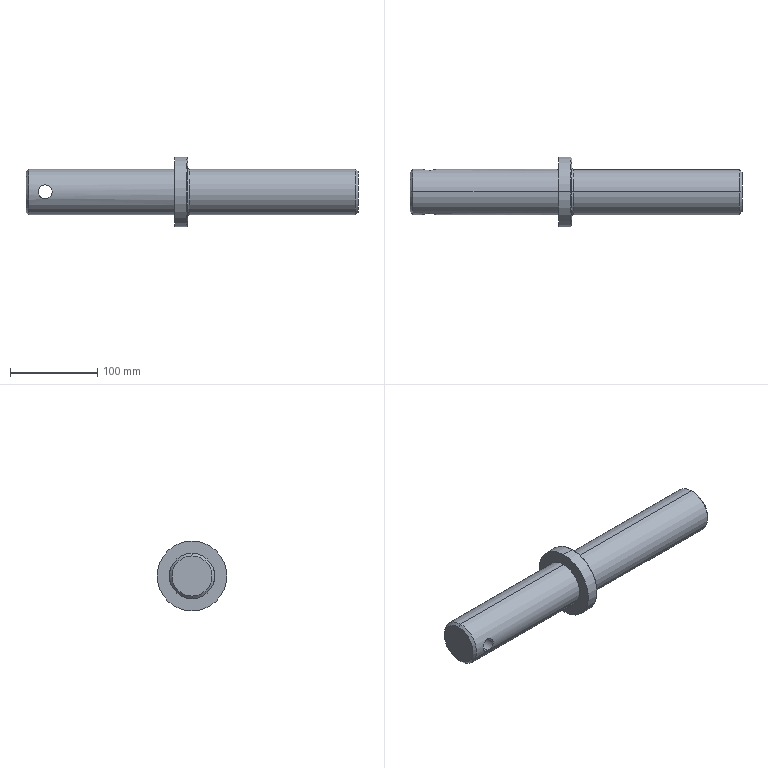Part | NX | features BREP 1 | 1 solid | 20 faces | box 380 x 80 x 80 mm | volume 838833 mm3 | cylinder 8 | cone 6 | plane 4 | torus 2 | commonest cylinder face diameters 52 x4 16 x2 80 x2
STEP:
#1=CARTESIAN_POINT('',(22.,-24.787,-7.85));
#2=VERTEX_POINT('',#1);
#3=CARTESIAN_POINT('',(22.,-24.689,8.15));
#4=VERTEX_POINT('',#3);
#5=CARTESIAN_POINT('',(22.,-24.787,-7.85));
#6=CARTESIAN_POINT('',(19.872,-24.787,-7.85));
#7=CARTESIAN_POINT('',(15.748,-25.421,-6.116));
#8=CARTESIAN_POINT('',(13.125,-26.307,0.145));
#9=CARTESIAN_POINT('',(15.749,-25.348,6.42));
#10=CARTESIAN_POINT('',(19.872,-24.689,8.15));
#11=CARTESIAN_POINT('',(22.,-24.689,8.15));
#12=B_SPLINE_CURVE_WITH_KNOTS('',3,(#5,#6,#7,#8,#9,#10,#11),.UNSPECIFIED.,.F.,.F.,(4,1,1,1,4),(0.,0.006289,0.01258,0.01887,0.02516),.UNSPECIFIED.);
#13=EDGE_CURVE('',#2,#4,#12,.T.);
#14=ORIENTED_EDGE('',*,*,#13,.F.);
#15=CARTESIAN_POINT('',(22.,24.787,-7.85));
#16=VERTEX_POINT('',#15);
#17=CARTESIAN_POINT('',(22.,-50.,-7.85));
#18=DIRECTION('',(0.,1.,0.));
#19=VECTOR('',#18,1000.);
#20=LINE('',#17,#19);
#21=EDGE_CURVE('',#2,#16,#20,.T.);
#22=ORIENTED_EDGE('',*,*,#21,.T.);
#23=CARTESIAN_POINT('',(22.,24.689,8.15));
#24=VERTEX_POINT('',#23);
#25=CARTESIAN_POINT('',(22.,24.689,8.15));
#26=CARTESIAN_POINT('',(19.872,24.689,8.15));
#27=CARTESIAN_POINT('',(15.753,25.347,6.416));
#28=CARTESIAN_POINT('',(13.126,26.307,0.1709));
#29=CARTESIAN_POINT('',(15.744,25.422,-6.119));
#30=CARTESIAN_POINT('',(19.872,24.787,-7.85));
#31=CARTESIAN_POINT('',(22.,24.787,-7.85));
#32=B_SPLINE_CURVE_WITH_KNOTS('',3,(#25,#26,#27,#28,#29,#30,#31),.UNSPECIFIED.,.F.,.F.,(4,1,1,1,4),(0.,0.006289,0.01258,0.01887,0.02516),.UNSPECIFIED.);
#33=EDGE_CURVE('',#24,#16,#32,.T.);
#34=ORIENTED_EDGE('',*,*,#33,.F.);
#35=CARTESIAN_POINT('',(22.,-50.,8.15));
#36=DIRECTION('',(0.,1.,0.));
#37=VECTOR('',#36,1000.);
#38=LINE('',#35,#37);
#39=EDGE_CURVE('',#4,#24,#38,.T.);
#40=ORIENTED_EDGE('',*,*,#39,.F.);
#41=EDGE_LOOP('',(#14,#22,#34,#40));
#42=FACE_BOUND('',#41,.T.);
#43=CARTESIAN_POINT('',(22.,-50.,0.1503));
#44=DIRECTION('',(0.,1.,0.));
#45=DIRECTION('',(0.,0.,-1.));
#46=AXIS2_PLACEMENT_3D('',#43,#44,#45);
#47=CYLINDRICAL_SURFACE('',#46,8.);
#48=ADVANCED_FACE('',(#42),#47,.F.);
#49=CARTESIAN_POINT('',(380.,0.,-23.));
#50=VERTEX_POINT('',#49);
#51=CARTESIAN_POINT('',(380.,0.,23.));
#52=VERTEX_POINT('',#51);
#53=CARTESIAN_POINT('',(380.,0.,0.));
#54=DIRECTION('',(1.,0.,0.));
#55=DIRECTION('',(0.,0.,1.));
#56=AXIS2_PLACEMENT_3D('',#53,#54,#55);
#57=CIRCLE('',#56,23.);
#58=EDGE_CURVE('',#50,#52,#57,.T.);
#59=ORIENTED_EDGE('',*,*,#58,.F.);
#60=CARTESIAN_POINT('',(377.,0.,-26.));
#61=VERTEX_POINT('',#60);
#62=CARTESIAN_POINT('',(377.,0.,-26.));
#63=DIRECTION('',(-0.7071,0.,-0.7071));
#64=VECTOR('',#63,1000.);
#65=LINE('',#62,#64);
#66=EDGE_CURVE('',#50,#61,#65,.T.);
#67=ORIENTED_EDGE('',*,*,#66,.T.);
#68=CARTESIAN_POINT('',(377.,0.,26.));
#69=VERTEX_POINT('',#68);
#70=CARTESIAN_POINT('',(377.,0.,0.));
#71=DIRECTION('',(-1.,0.,0.));
#72=DIRECTION('',(0.,0.,1.));
#73=AXIS2_PLACEMENT_3D('',#70,#71,#72);
#74=CIRCLE('',#73,26.);
#75=EDGE_CURVE('',#69,#61,#74,.T.);
#76=ORIENTED_EDGE('',*,*,#75,.F.);
#77=CARTESIAN_POINT('',(377.,0.,26.));
#78=DIRECTION('',(-0.7071,0.,0.7071));
#79=VECTOR('',#78,1000.);
#80=LINE('',#77,#79);
#81=EDGE_CURVE('',#52,#69,#80,.T.);
#82=ORIENTED_EDGE('',*,*,#81,.F.);
#83=EDGE_LOOP('',(#59,#67,#76,#82));
#84=FACE_BOUND('',#83,.T.);
#85=CARTESIAN_POINT('',(377.,0.,0.));
#86=DIRECTION('',(-1.,0.,0.));
#87=DIRECTION('',(0.,0.,-1.));
#88=AXIS2_PLACEMENT_3D('',#85,#86,#87);
#89=CONICAL_SURFACE('',#88,26.,0.7854);
#90=ADVANCED_FACE('',(#84),#89,.T.);
#91=CARTESIAN_POINT('',(0.,0.,23.));
#92=VERTEX_POINT('',#91);
#93=CARTESIAN_POINT('',(0.,0.,-23.));
#94=VERTEX_POINT('',#93);
#95=CARTESIAN_POINT('',(0.,0.,0.));
#96=DIRECTION('',(-1.,0.,0.));
#97=DIRECTION('',(0.,0.,-1.));
#98=AXIS2_PLACEMENT_3D('',#95,#96,#97);
#99=CIRCLE('',#98,23.);
#100=EDGE_CURVE('',#92,#94,#99,.T.);
#101=ORIENTED_EDGE('',*,*,#100,.F.);
#102=CARTESIAN_POINT('',(3.,0.,26.));
#103=VERTEX_POINT('',#102);
#104=CARTESIAN_POINT('',(0.,0.,23.));
#105=DIRECTION('',(0.7071,0.,0.7071));
#106=VECTOR('',#105,1000.);
#107=LINE('',#104,#106);
#108=EDGE_CURVE('',#103,#92,#107,.F.);
#109=ORIENTED_EDGE('',*,*,#108,.F.);
#110=CARTESIAN_POINT('',(3.,0.,-26.));
#111=VERTEX_POINT('',#110);
#112=CARTESIAN_POINT('',(3.,0.,0.));
#113=DIRECTION('',(1.,0.,0.));
#114=DIRECTION('',(0.,0.,-1.));
#115=AXIS2_PLACEMENT_3D('',#112,#113,#114);
#116=CIRCLE('',#115,26.);
#117=EDGE_CURVE('',#111,#103,#116,.T.);
#118=ORIENTED_EDGE('',*,*,#117,.F.);
#119=CARTESIAN_POINT('',(0.,0.,-23.));
#120=DIRECTION('',(0.7071,0.,-0.7071));
#121=VECTOR('',#120,1000.);
#122=LINE('',#119,#121);
#123=EDGE_CURVE('',#111,#94,#122,.F.);
#124=ORIENTED_EDGE('',*,*,#123,.T.);
#125=EDGE_LOOP('',(#101,#109,#118,#124));
#126=FACE_BOUND('',#125,.T.);
#127=CARTESIAN_POINT('',(0.,0.,0.));
#128=DIRECTION('',(1.,0.,0.));
#129=DIRECTION('',(0.,0.,1.));
#130=AXIS2_PLACEMENT_3D('',#127,#128,#129);
#131=CONICAL_SURFACE('',#130,23.,0.7854);
#132=ADVANCED_FACE('',(#126),#131,.T.);
#133=CARTESIAN_POINT('',(185.,0.,-28.));
#134=VERTEX_POINT('',#133);
#135=CARTESIAN_POINT('',(185.,0.,28.));
#136=VERTEX_POINT('',#135);
#137=CARTESIAN_POINT('',(185.,0.,0.));
#138=DIRECTION('',(-1.,0.,0.));
#139=DIRECTION('',(0.,0.,1.));
#140=AXIS2_PLACEMENT_3D('',#137,#138,#139);
#141=CIRCLE('',#140,28.);
#142=EDGE_CURVE('',#134,#136,#141,.T.);
#143=ORIENTED_EDGE('',*,*,#142,.F.);
#144=CARTESIAN_POINT('',(187.,0.,-26.));
#145=VERTEX_POINT('',#144);
#146=CARTESIAN_POINT('',(187.,0.,-28.));
#147=DIRECTION('',(0.,1.,0.));
#148=DIRECTION('',(0.,0.,1.));
#149=AXIS2_PLACEMENT_3D('',#146,#147,#148);
#150=CIRCLE('',#149,2.);
#151=EDGE_CURVE('',#134,#145,#150,.T.);
#152=ORIENTED_EDGE('',*,*,#151,.T.);
#153=CARTESIAN_POINT('',(187.,0.,26.));
#154=VERTEX_POINT('',#153);
#155=CARTESIAN_POINT('',(187.,0.,0.));
#156=DIRECTION('',(1.,0.,0.));
#157=DIRECTION('',(0.,0.,1.));
#158=AXIS2_PLACEMENT_3D('',#155,#156,#157);
#159=CIRCLE('',#158,26.);
#160=EDGE_CURVE('',#154,#145,#159,.T.);
#161=ORIENTED_EDGE('',*,*,#160,.F.);
#162=CARTESIAN_POINT('',(187.,0.,28.));
#163=DIRECTION('',(0.,-1.,0.));
#164=DIRECTION('',(0.,0.,-1.));
#165=AXIS2_PLACEMENT_3D('',#162,#163,#164);
#166=CIRCLE('',#165,2.);
#167=EDGE_CURVE('',#136,#154,#166,.T.);
#168=ORIENTED_EDGE('',*,*,#167,.F.);
#169=EDGE_LOOP('',(#143,#152,#161,#168));
#170=FACE_BOUND('',#169,.T.);
#171=CARTESIAN_POINT('',(187.,0.,0.));
#172=DIRECTION('',(-1.,0.,0.));
#173=DIRECTION('',(0.,0.,-1.));
#174=AXIS2_PLACEMENT_3D('',#171,#172,#173);
#175=TOROIDAL_SURFACE('',#174,28.,2.);
#176=ADVANCED_FACE('',(#170),#175,.F.);
#177=CARTESIAN_POINT('',(185.,0.,-39.));
#178=VERTEX_POINT('',#177);
#179=CARTESIAN_POINT('',(185.,0.,39.));
#180=VERTEX_POINT('',#179);
#181=CARTESIAN_POINT('',(185.,0.,0.));
#182=DIRECTION('',(1.,0.,0.));
#183=DIRECTION('',(0.,0.,1.));
#184=AXIS2_PLACEMENT_3D('',#181,#182,#183);
#185=CIRCLE('',#184,39.);
#186=EDGE_CURVE('',#178,#180,#185,.T.);
#187=ORIENTED_EDGE('',*,*,#186,.F.);
#188=CARTESIAN_POINT('',(184.,0.,-40.));
#189=VERTEX_POINT('',#188);
#190=CARTESIAN_POINT('',(184.,0.,-40.));
#191=DIRECTION('',(-0.7071,0.,-0.7071));
#192=VECTOR('',#191,1000.);
#193=LINE('',#190,#192);
#194=EDGE_CURVE('',#178,#189,#193,.T.);
#195=ORIENTED_EDGE('',*,*,#194,.T.);
#196=CARTESIAN_POINT('',(184.,0.,40.));
#197=VERTEX_POINT('',#196);
#198=CARTESIAN_POINT('',(184.,0.,0.));
#199=DIRECTION('',(-1.,0.,0.));
#200=DIRECTION('',(0.,0.,1.));
#201=AXIS2_PLACEMENT_3D('',#198,#199,#200);
#202=CIRCLE('',#201,40.);
#203=EDGE_CURVE('',#197,#189,#202,.T.);
#204=ORIENTED_EDGE('',*,*,#203,.F.);
#205=CARTESIAN_POINT('',(184.,0.,40.));
#206=DIRECTION('',(-0.7071,0.,0.7071));
#207=VECTOR('',#206,1000.);
#208=LINE('',#205,#207);
#209=EDGE_CURVE('',#180,#197,#208,.T.);
#210=ORIENTED_EDGE('',*,*,#209,.F.);
#211=EDGE_LOOP('',(#187,#195,#204,#210));
#212=FACE_BOUND('',#211,.T.);
#213=CARTESIAN_POINT('',(184.,0.,0.));
#214=DIRECTION('',(-1.,0.,0.));
#215=DIRECTION('',(0.,0.,-1.));
#216=AXIS2_PLACEMENT_3D('',#213,#214,#215);
#217=CONICAL_SURFACE('',#216,40.,0.7854);
#218=ADVANCED_FACE('',(#212),#217,.T.);
#219=ORIENTED_EDGE('',*,*,#33,.T.);
#220=CARTESIAN_POINT('',(22.,24.787,-7.85));
#221=CARTESIAN_POINT('',(24.128,24.787,-7.85));
#222=CARTESIAN_POINT('',(28.252,25.421,-6.116));
#223=CARTESIAN_POINT('',(30.875,26.307,0.145));
#224=CARTESIAN_POINT('',(28.251,25.348,6.42));
#225=CARTESIAN_POINT('',(24.128,24.689,8.15));
#226=CARTESIAN_POINT('',(22.,24.689,8.15));
#227=B_SPLINE_CURVE_WITH_KNOTS('',3,(#220,#221,#222,#223,#224,#225,#226),.UNSPECIFIED.,.F.,.F.,(4,1,1,1,4),(0.,0.006289,0.01258,0.01887,0.02516),.UNSPECIFIED.);
#228=EDGE_CURVE('',#16,#24,#227,.T.);
#229=ORIENTED_EDGE('',*,*,#228,.T.);
#230=EDGE_LOOP('',(#219,#229));
#231=FACE_BOUND('',#230,.T.);
#232=CARTESIAN_POINT('',(170.,0.,26.));
#233=VERTEX_POINT('',#232);
#234=CARTESIAN_POINT('',(170.,0.,-26.));
#235=VERTEX_POINT('',#234);
#236=CARTESIAN_POINT('',(170.,0.,0.));
#237=DIRECTION('',(-1.,0.,0.));
#238=DIRECTION('',(0.,0.,1.));
#239=AXIS2_PLACEMENT_3D('',#236,#237,#238);
#240=CIRCLE('',#239,26.);
#241=EDGE_CURVE('',#233,#235,#240,.T.);
#242=ORIENTED_EDGE('',*,*,#241,.T.);
#243=CARTESIAN_POINT('',(0.,0.,-26.));
#244=DIRECTION('',(-1.,0.,0.));
#245=VECTOR('',#244,1000.);
#246=LINE('',#243,#245);
#247=EDGE_CURVE('',#235,#111,#246,.T.);
#248=ORIENTED_EDGE('',*,*,#247,.T.);
#249=ORIENTED_EDGE('',*,*,#117,.T.);
#250=CARTESIAN_POINT('',(0.,0.,26.));
#251=DIRECTION('',(-1.,0.,0.));
#252=VECTOR('',#251,1000.);
#253=LINE('',#250,#252);
#254=EDGE_CURVE('',#233,#103,#253,.T.);
#255=ORIENTED_EDGE('',*,*,#254,.F.);
#256=EDGE_LOOP('',(#242,#248,#249,#255));
#257=FACE_BOUND('',#256,.T.);
#258=CARTESIAN_POINT('',(0.,0.,0.));
#259=DIRECTION('',(-1.,0.,0.));
#260=DIRECTION('',(0.,0.,-1.));
#261=AXIS2_PLACEMENT_3D('',#258,#259,#260);
#262=CYLINDRICAL_SURFACE('',#261,26.);
#263=ADVANCED_FACE('',(#231,#257),#262,.T.);
#264=ORIENTED_EDGE('',*,*,#203,.T.);
#265=CARTESIAN_POINT('',(170.,0.,-40.));
#266=VERTEX_POINT('',#265);
#267=CARTESIAN_POINT('',(0.,0.,-40.));
#268=DIRECTION('',(-1.,0.,0.));
#269=VECTOR('',#268,1000.);
#270=LINE('',#267,#269);
#271=EDGE_CURVE('',#189,#266,#270,.T.);
#272=ORIENTED_EDGE('',*,*,#271,.T.);
#273=CARTESIAN_POINT('',(170.,0.,40.));
#274=VERTEX_POINT('',#273);
#275=CARTESIAN_POINT('',(170.,0.,0.));
#276=DIRECTION('',(-1.,0.,0.));
#277=DIRECTION('',(0.,0.,1.));
#278=AXIS2_PLACEMENT_3D('',#275,#276,#277);
#279=CIRCLE('',#278,40.);
#280=EDGE_CURVE('',#274,#266,#279,.T.);
#281=ORIENTED_EDGE('',*,*,#280,.F.);
#282=CARTESIAN_POINT('',(0.,0.,40.));
#283=DIRECTION('',(-1.,0.,0.));
#284=VECTOR('',#283,1000.);
#285=LINE('',#282,#284);
#286=EDGE_CURVE('',#197,#274,#285,.T.);
#287=ORIENTED_EDGE('',*,*,#286,.F.);
#288=EDGE_LOOP('',(#264,#272,#281,#287));
#289=FACE_BOUND('',#288,.T.);
#290=CARTESIAN_POINT('',(0.,0.,0.));
#291=DIRECTION('',(-1.,0.,0.));
#292=DIRECTION('',(0.,0.,-1.));
#293=AXIS2_PLACEMENT_3D('',#290,#291,#292);
#294=CYLINDRICAL_SURFACE('',#293,40.);
#295=ADVANCED_FACE('',(#289),#294,.T.);
#296=ORIENTED_EDGE('',*,*,#75,.T.);
#297=CARTESIAN_POINT('',(0.,0.,-26.));
#298=DIRECTION('',(-1.,0.,0.));
#299=VECTOR('',#298,1000.);
#300=LINE('',#297,#299);
#301=EDGE_CURVE('',#61,#145,#300,.T.);
#302=ORIENTED_EDGE('',*,*,#301,.T.);
#303=CARTESIAN_POINT('',(187.,0.,0.));
#304=DIRECTION('',(1.,0.,0.));
#305=DIRECTION('',(0.,0.,1.));
#306=AXIS2_PLACEMENT_3D('',#303,#304,#305);
#307=CIRCLE('',#306,26.);
#308=EDGE_CURVE('',#145,#154,#307,.T.);
#309=ORIENTED_EDGE('',*,*,#308,.T.);
#310=CARTESIAN_POINT('',(0.,0.,26.));
#311=DIRECTION('',(-1.,0.,0.));
#312=VECTOR('',#311,1000.);
#313=LINE('',#310,#312);
#314=EDGE_CURVE('',#69,#154,#313,.T.);
#315=ORIENTED_EDGE('',*,*,#314,.F.);
#316=EDGE_LOOP('',(#296,#302,#309,#315));
#317=FACE_BOUND('',#316,.T.);
#318=CARTESIAN_POINT('',(0.,0.,0.));
#319=DIRECTION('',(-1.,0.,0.));
#320=DIRECTION('',(0.,0.,-1.));
#321=AXIS2_PLACEMENT_3D('',#318,#319,#320);
#322=CYLINDRICAL_SURFACE('',#321,26.);
#323=ADVANCED_FACE('',(#317),#322,.T.);
#324=CARTESIAN_POINT('',(0.,0.,0.));
#325=DIRECTION('',(-1.,0.,0.));
#326=DIRECTION('',(0.,0.,-1.));
#327=AXIS2_PLACEMENT_3D('',#324,#325,#326);
#328=CIRCLE('',#327,23.);
#329=EDGE_CURVE('',#94,#92,#328,.T.);
#330=ORIENTED_EDGE('',*,*,#329,.T.);
#331=ORIENTED_EDGE('',*,*,#100,.T.);
#332=EDGE_LOOP('',(#330,#331));
#333=FACE_BOUND('',#332,.T.);
#334=CARTESIAN_POINT('',(0.,26.,0.));
#335=DIRECTION('',(1.,0.,0.));
#336=DIRECTION('',(0.,0.,1.));
#337=AXIS2_PLACEMENT_3D('',#334,#335,#336);
#338=PLANE('',#337);
#339=ADVANCED_FACE('',(#333),#338,.F.);
#340=CARTESIAN_POINT('',(380.,0.,0.));
#341=DIRECTION('',(1.,0.,0.));
#342=DIRECTION('',(0.,0.,1.));
#343=AXIS2_PLACEMENT_3D('',#340,#341,#342);
#344=CIRCLE('',#343,23.);
#345=EDGE_CURVE('',#52,#50,#344,.T.);
#346=ORIENTED_EDGE('',*,*,#345,.T.);
#347=ORIENTED_EDGE('',*,*,#58,.T.);
#348=EDGE_LOOP('',(#346,#347));
#349=FACE_BOUND('',#348,.T.);
#350=CARTESIAN_POINT('',(380.,0.,0.));
#351=DIRECTION('',(-1.,0.,0.));
#352=DIRECTION('',(0.,0.,-1.));
#353=AXIS2_PLACEMENT_3D('',#350,#351,#352);
#354=PLANE('',#353);
#355=ADVANCED_FACE('',(#349),#354,.F.);
#356=ORIENTED_EDGE('',*,*,#301,.F.);
#357=CARTESIAN_POINT('',(377.,0.,0.));
#358=DIRECTION('',(-1.,0.,0.));
#359=DIRECTION('',(0.,0.,1.));
#360=AXIS2_PLACEMENT_3D('',#357,#358,#359);
#361=CIRCLE('',#360,26.);
#362=EDGE_CURVE('',#61,#69,#361,.T.);
#363=ORIENTED_EDGE('',*,*,#362,.T.);
#364=ORIENTED_EDGE('',*,*,#314,.T.);
#365=ORIENTED_EDGE('',*,*,#160,.T.);
#366=EDGE_LOOP('',(#356,#363,#364,#365));
#367=FACE_BOUND('',#366,.T.);
#368=CARTESIAN_POINT('',(0.,0.,0.));
#369=DIRECTION('',(-1.,0.,0.));
#370=DIRECTION('',(0.,0.,-1.));
#371=AXIS2_PLACEMENT_3D('',#368,#369,#370);
#372=CYLINDRICAL_SURFACE('',#371,26.);
#373=ADVANCED_FACE('',(#367),#372,.T.);
#374=CARTESIAN_POINT('',(185.,0.,0.));
#375=DIRECTION('',(-1.,0.,0.));
#376=DIRECTION('',(0.,0.,1.));
#377=AXIS2_PLACEMENT_3D('',#374,#375,#376);
#378=CIRCLE('',#377,28.);
#379=EDGE_CURVE('',#136,#134,#378,.T.);
#380=ORIENTED_EDGE('',*,*,#379,.T.);
#381=ORIENTED_EDGE('',*,*,#142,.T.);
#382=EDGE_LOOP('',(#380,#381));
#383=FACE_BOUND('',#382,.T.);
#384=CARTESIAN_POINT('',(185.,0.,0.));
#385=DIRECTION('',(1.,0.,0.));
#386=DIRECTION('',(0.,0.,1.));
#387=AXIS2_PLACEMENT_3D('',#384,#385,#386);
#388=CIRCLE('',#387,39.);
#389=EDGE_CURVE('',#180,#178,#388,.T.);
#390=ORIENTED_EDGE('',*,*,#389,.T.);
#391=ORIENTED_EDGE('',*,*,#186,.T.);
#392=EDGE_LOOP('',(#390,#391));
#393=FACE_BOUND('',#392,.T.);
#394=CARTESIAN_POINT('',(185.,26.,0.));
#395=DIRECTION('',(-1.,0.,0.));
#396=DIRECTION('',(0.,0.,-1.));
#397=AXIS2_PLACEMENT_3D('',#394,#395,#396);
#398=PLANE('',#397);
#399=ADVANCED_FACE('',(#383,#393),#398,.F.);
#400=ORIENTED_EDGE('',*,*,#271,.F.);
#401=CARTESIAN_POINT('',(184.,0.,0.));
#402=DIRECTION('',(-1.,0.,0.));
#403=DIRECTION('',(0.,0.,1.));
#404=AXIS2_PLACEMENT_3D('',#401,#402,#403);
#405=CIRCLE('',#404,40.);
#406=EDGE_CURVE('',#189,#197,#405,.T.);
#407=ORIENTED_EDGE('',*,*,#406,.T.);
#408=ORIENTED_EDGE('',*,*,#286,.T.);
#409=CARTESIAN_POINT('',(170.,0.,0.));
#410=DIRECTION('',(-1.,0.,0.));
#411=DIRECTION('',(0.,0.,1.));
#412=AXIS2_PLACEMENT_3D('',#409,#410,#411);
#413=CIRCLE('',#412,40.);
#414=EDGE_CURVE('',#266,#274,#413,.T.);
#415=ORIENTED_EDGE('',*,*,#414,.F.);
#416=EDGE_LOOP('',(#400,#407,#408,#415));
#417=FACE_BOUND('',#416,.T.);
#418=CARTESIAN_POINT('',(0.,0.,0.));
#419=DIRECTION('',(-1.,0.,0.));
#420=DIRECTION('',(0.,0.,-1.));
#421=AXIS2_PLACEMENT_3D('',#418,#419,#420);
#422=CYLINDRICAL_SURFACE('',#421,40.);
#423=ADVANCED_FACE('',(#417),#422,.T.);
#424=ORIENTED_EDGE('',*,*,#241,.F.);
#425=CARTESIAN_POINT('',(170.,0.,0.));
#426=DIRECTION('',(-1.,0.,0.));
#427=DIRECTION('',(0.,0.,1.));
#428=AXIS2_PLACEMENT_3D('',#425,#426,#427);
#429=CIRCLE('',#428,26.);
#430=EDGE_CURVE('',#235,#233,#429,.T.);
#431=ORIENTED_EDGE('',*,*,#430,.F.);
#432=EDGE_LOOP('',(#424,#431));
#433=FACE_BOUND('',#432,.T.);
#434=ORIENTED_EDGE('',*,*,#280,.T.);
#435=ORIENTED_EDGE('',*,*,#414,.T.);
#436=EDGE_LOOP('',(#434,#435));
#437=FACE_BOUND('',#436,.T.);
#438=CARTESIAN_POINT('',(170.,40.,0.));
#439=DIRECTION('',(1.,0.,0.));
#440=DIRECTION('',(0.,0.,1.));
#441=AXIS2_PLACEMENT_3D('',#438,#439,#440);
#442=PLANE('',#441);
#443=ADVANCED_FACE('',(#433,#437),#442,.F.);
#444=ORIENTED_EDGE('',*,*,#247,.F.);
#445=ORIENTED_EDGE('',*,*,#430,.T.);
#446=ORIENTED_EDGE('',*,*,#254,.T.);
#447=CARTESIAN_POINT('',(3.,0.,0.));
#448=DIRECTION('',(1.,0.,0.));
#449=DIRECTION('',(0.,0.,-1.));
#450=AXIS2_PLACEMENT_3D('',#447,#448,#449);
#451=CIRCLE('',#450,26.);
#452=EDGE_CURVE('',#103,#111,#451,.T.);
#453=ORIENTED_EDGE('',*,*,#452,.T.);
#454=EDGE_LOOP('',(#444,#445,#446,#453));
#455=FACE_BOUND('',#454,.T.);
#456=CARTESIAN_POINT('',(22.,-24.689,8.15));
#457=CARTESIAN_POINT('',(24.128,-24.689,8.15));
#458=CARTESIAN_POINT('',(28.247,-25.347,6.416));
#459=CARTESIAN_POINT('',(30.874,-26.307,0.1709));
#460=CARTESIAN_POINT('',(28.256,-25.422,-6.119));
#461=CARTESIAN_POINT('',(24.128,-24.787,-7.85));
#462=CARTESIAN_POINT('',(22.,-24.787,-7.85));
#463=B_SPLINE_CURVE_WITH_KNOTS('',3,(#456,#457,#458,#459,#460,#461,#462),.UNSPECIFIED.,.F.,.F.,(4,1,1,1,4),(0.,0.006289,0.01258,0.01887,0.02516),.UNSPECIFIED.);
#464=EDGE_CURVE('',#4,#2,#463,.T.);
#465=ORIENTED_EDGE('',*,*,#464,.T.);
#466=ORIENTED_EDGE('',*,*,#13,.T.);
#467=EDGE_LOOP('',(#465,#466));
#468=FACE_BOUND('',#467,.T.);
#469=CARTESIAN_POINT('',(0.,0.,0.));
#470=DIRECTION('',(-1.,0.,0.));
#471=DIRECTION('',(0.,0.,-1.));
#472=AXIS2_PLACEMENT_3D('',#469,#470,#471);
#473=CYLINDRICAL_SURFACE('',#472,26.);
#474=ADVANCED_FACE('',(#455,#468),#473,.T.);
#475=ORIENTED_EDGE('',*,*,#194,.F.);
#476=ORIENTED_EDGE('',*,*,#389,.F.);
#477=ORIENTED_EDGE('',*,*,#209,.T.);
#478=ORIENTED_EDGE('',*,*,#406,.F.);
#479=EDGE_LOOP('',(#475,#476,#477,#478));
#480=FACE_BOUND('',#479,.T.);
#481=CARTESIAN_POINT('',(184.,0.,0.));
#482=DIRECTION('',(-1.,0.,0.));
#483=DIRECTION('',(0.,0.,-1.));
#484=AXIS2_PLACEMENT_3D('',#481,#482,#483);
#485=CONICAL_SURFACE('',#484,40.,0.7854);
#486=ADVANCED_FACE('',(#480),#485,.T.);
#487=ORIENTED_EDGE('',*,*,#151,.F.);
#488=ORIENTED_EDGE('',*,*,#379,.F.);
#489=ORIENTED_EDGE('',*,*,#167,.T.);
#490=ORIENTED_EDGE('',*,*,#308,.F.);
#491=EDGE_LOOP('',(#487,#488,#489,#490));
#492=FACE_BOUND('',#491,.T.);
#493=CARTESIAN_POINT('',(187.,0.,0.));
#494=DIRECTION('',(-1.,0.,0.));
#495=DIRECTION('',(0.,0.,-1.));
#496=AXIS2_PLACEMENT_3D('',#493,#494,#495);
#497=TOROIDAL_SURFACE('',#496,28.,2.);
#498=ADVANCED_FACE('',(#492),#497,.F.);
#499=ORIENTED_EDGE('',*,*,#108,.T.);
#500=ORIENTED_EDGE('',*,*,#329,.F.);
#501=ORIENTED_EDGE('',*,*,#123,.F.);
#502=ORIENTED_EDGE('',*,*,#452,.F.);
#503=EDGE_LOOP('',(#499,#500,#501,#502));
#504=FACE_BOUND('',#503,.T.);
#505=CARTESIAN_POINT('',(0.,0.,0.));
#506=DIRECTION('',(1.,0.,0.));
#507=DIRECTION('',(0.,0.,1.));
#508=AXIS2_PLACEMENT_3D('',#505,#506,#507);
#509=CONICAL_SURFACE('',#508,23.,0.7854);
#510=ADVANCED_FACE('',(#504),#509,.T.);
#511=ORIENTED_EDGE('',*,*,#66,.F.);
#512=ORIENTED_EDGE('',*,*,#345,.F.);
#513=ORIENTED_EDGE('',*,*,#81,.T.);
#514=ORIENTED_EDGE('',*,*,#362,.F.);
#515=EDGE_LOOP('',(#511,#512,#513,#514));
#516=FACE_BOUND('',#515,.T.);
#517=CARTESIAN_POINT('',(377.,0.,0.));
#518=DIRECTION('',(-1.,0.,0.));
#519=DIRECTION('',(0.,0.,-1.));
#520=AXIS2_PLACEMENT_3D('',#517,#518,#519);
#521=CONICAL_SURFACE('',#520,26.,0.7854);
#522=ADVANCED_FACE('',(#516),#521,.T.);
#523=ORIENTED_EDGE('',*,*,#21,.F.);
#524=ORIENTED_EDGE('',*,*,#464,.F.);
#525=ORIENTED_EDGE('',*,*,#39,.T.);
#526=ORIENTED_EDGE('',*,*,#228,.F.);
#527=EDGE_LOOP('',(#523,#524,#525,#526));
#528=FACE_BOUND('',#527,.T.);
#529=CARTESIAN_POINT('',(22.,-50.,0.1503));
#530=DIRECTION('',(0.,1.,0.));
#531=DIRECTION('',(0.,0.,-1.));
#532=AXIS2_PLACEMENT_3D('',#529,#530,#531);
#533=CYLINDRICAL_SURFACE('',#532,8.);
#534=ADVANCED_FACE('',(#528),#533,.F.);
#535=CLOSED_SHELL('',(#48,#90,#132,#176,#218,#263,#295,#323,#339,#355,#373,#399,#423,#443,#474,#486,#498,#510,#522,#534));
#536=MANIFOLD_SOLID_BREP('',#535);
#537=(LENGTH_UNIT()NAMED_UNIT(*)SI_UNIT(.MILLI.,.METRE.));
#538=UNCERTAINTY_MEASURE_WITH_UNIT(LENGTH_MEASURE(0.0508),#537,'','');
#539=(NAMED_UNIT(*)PLANE_ANGLE_UNIT()SI_UNIT($,.RADIAN.));
#540=(NAMED_UNIT(*)SI_UNIT($,.STERADIAN.)SOLID_ANGLE_UNIT());
#541=(GEOMETRIC_REPRESENTATION_CONTEXT(3)GLOBAL_UNCERTAINTY_ASSIGNED_CONTEXT((#538))GLOBAL_UNIT_ASSIGNED_CONTEXT((#537,#539,#540))REPRESENTATION_CONTEXT('',''));
#542=ADVANCED_BREP_SHAPE_REPRESENTATION('',(#536),#541);